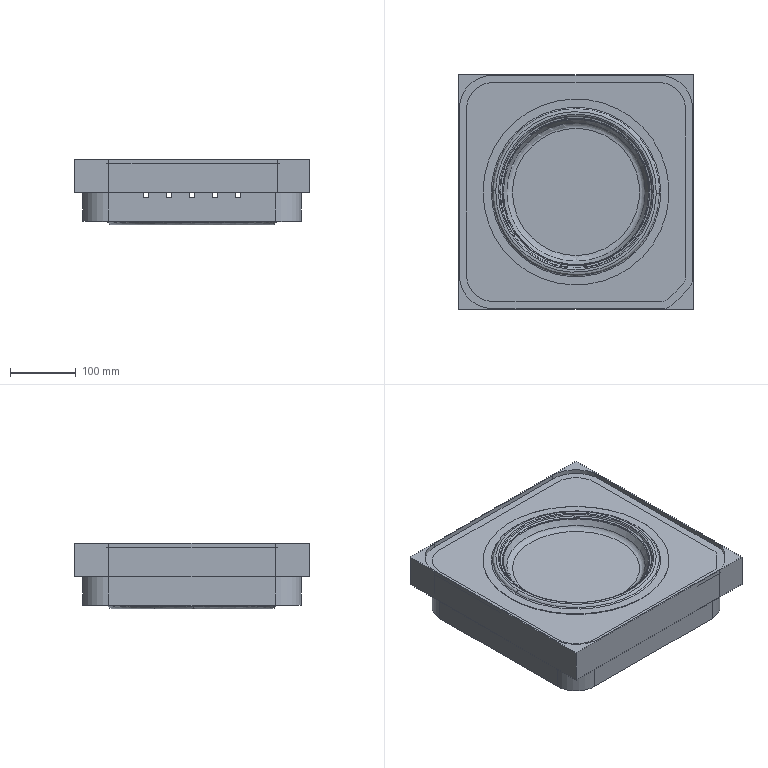Part | 4 solids | 449 faces | box 356 x 356 x 99.5 mm | volume 9185531 mm3 | plane 200 | cylinder 197 | spline 44 | cone 4 | torus 4 | commonest cylinder face diameters 2 x87 8 x33 178.502 x10 195.102 x10 80 x9 145.102 x8